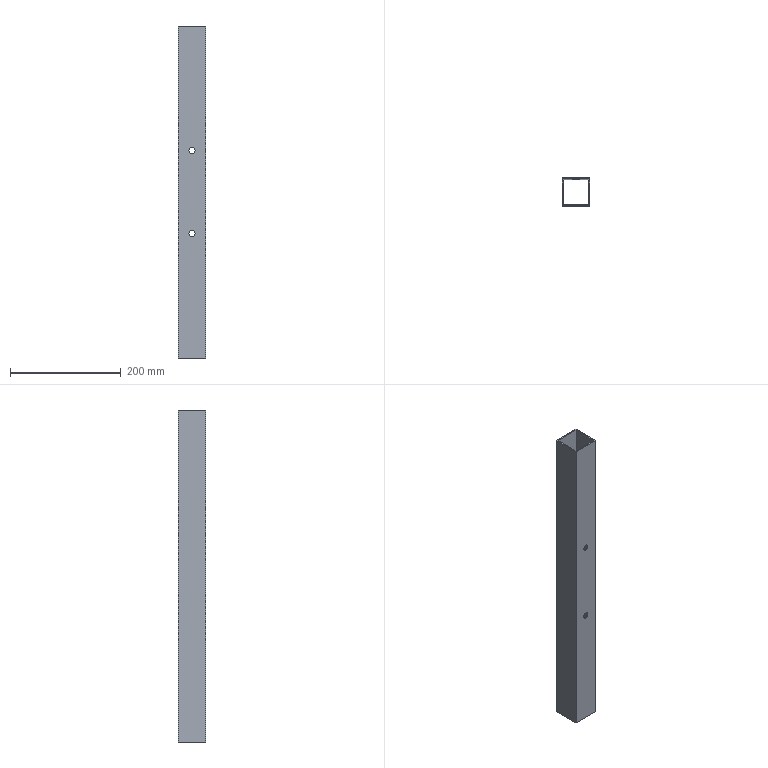Part | SolidWorks | features Cut 1, Extrusion 1 | 1 solid | 18 faces | box 50 x 50 x 600 mm | volume 229640 mm3 | plane 10 | cylinder 8 | commonest cylinder face diameters 11 x8
STEP:
#1=CARTESIAN_POINT('',(0.,23.,380.5));
#2=VERTEX_POINT('',#1);
#3=CARTESIAN_POINT('',(0.,23.,369.5));
#4=VERTEX_POINT('',#3);
#5=CARTESIAN_POINT('',(0.,23.,375.));
#6=DIRECTION('',(0.,-1.,0.));
#7=DIRECTION('',(0.,0.,-1.));
#8=AXIS2_PLACEMENT_3D('',#5,#6,#7);
#9=CIRCLE('',#8,5.5);
#10=EDGE_CURVE('',#2,#4,#9,.T.);
#11=ORIENTED_EDGE('',*,*,#10,.T.);
#12=CARTESIAN_POINT('',(0.,25.,369.5));
#13=VERTEX_POINT('',#12);
#14=CARTESIAN_POINT('',(0.,-25.,369.5));
#15=DIRECTION('',(0.,1.,0.));
#16=VECTOR('',#15,1000.);
#17=LINE('',#14,#16);
#18=EDGE_CURVE('',#4,#13,#17,.T.);
#19=ORIENTED_EDGE('',*,*,#18,.T.);
#20=CARTESIAN_POINT('',(0.,25.,380.5));
#21=VERTEX_POINT('',#20);
#22=CARTESIAN_POINT('',(0.,25.,375.));
#23=DIRECTION('',(0.,1.,0.));
#24=DIRECTION('',(0.,0.,1.));
#25=AXIS2_PLACEMENT_3D('',#22,#23,#24);
#26=CIRCLE('',#25,5.5);
#27=EDGE_CURVE('',#13,#21,#26,.T.);
#28=ORIENTED_EDGE('',*,*,#27,.T.);
#29=CARTESIAN_POINT('',(0.,-25.,380.5));
#30=DIRECTION('',(0.,1.,0.));
#31=VECTOR('',#30,1000.);
#32=LINE('',#29,#31);
#33=EDGE_CURVE('',#2,#21,#32,.T.);
#34=ORIENTED_EDGE('',*,*,#33,.F.);
#35=EDGE_LOOP('',(#11,#19,#28,#34));
#36=FACE_OUTER_BOUND('',#35,.T.);
#37=CARTESIAN_POINT('',(0.,-25.,375.));
#38=DIRECTION('',(0.,1.,0.));
#39=DIRECTION('',(0.,0.,1.));
#40=AXIS2_PLACEMENT_3D('',#37,#38,#39);
#41=CYLINDRICAL_SURFACE('',#40,5.5);
#42=ADVANCED_FACE('',(#36),#41,.F.);
#43=CARTESIAN_POINT('',(0.,-25.,369.5));
#44=VERTEX_POINT('',#43);
#45=CARTESIAN_POINT('',(0.,-25.,380.5));
#46=VERTEX_POINT('',#45);
#47=CARTESIAN_POINT('',(0.,-25.,375.));
#48=DIRECTION('',(0.,1.,0.));
#49=DIRECTION('',(0.,0.,1.));
#50=AXIS2_PLACEMENT_3D('',#47,#48,#49);
#51=CIRCLE('',#50,5.5);
#52=EDGE_CURVE('',#44,#46,#51,.T.);
#53=ORIENTED_EDGE('',*,*,#52,.F.);
#54=CARTESIAN_POINT('',(0.,-23.,369.5));
#55=VERTEX_POINT('',#54);
#56=CARTESIAN_POINT('',(0.,-25.,369.5));
#57=DIRECTION('',(0.,1.,0.));
#58=VECTOR('',#57,1000.);
#59=LINE('',#56,#58);
#60=EDGE_CURVE('',#44,#55,#59,.T.);
#61=ORIENTED_EDGE('',*,*,#60,.T.);
#62=CARTESIAN_POINT('',(0.,-23.,380.5));
#63=VERTEX_POINT('',#62);
#64=CARTESIAN_POINT('',(0.,-23.,375.));
#65=DIRECTION('',(0.,1.,0.));
#66=DIRECTION('',(0.,0.,1.));
#67=AXIS2_PLACEMENT_3D('',#64,#65,#66);
#68=CIRCLE('',#67,5.5);
#69=EDGE_CURVE('',#55,#63,#68,.T.);
#70=ORIENTED_EDGE('',*,*,#69,.T.);
#71=CARTESIAN_POINT('',(0.,-25.,380.5));
#72=DIRECTION('',(0.,1.,0.));
#73=VECTOR('',#72,1000.);
#74=LINE('',#71,#73);
#75=EDGE_CURVE('',#46,#63,#74,.T.);
#76=ORIENTED_EDGE('',*,*,#75,.F.);
#77=EDGE_LOOP('',(#53,#61,#70,#76));
#78=FACE_OUTER_BOUND('',#77,.T.);
#79=CARTESIAN_POINT('',(0.,-25.,375.));
#80=DIRECTION('',(0.,1.,0.));
#81=DIRECTION('',(0.,0.,1.));
#82=AXIS2_PLACEMENT_3D('',#79,#80,#81);
#83=CYLINDRICAL_SURFACE('',#82,5.5);
#84=ADVANCED_FACE('',(#78),#83,.F.);
#85=CARTESIAN_POINT('',(0.,23.,230.5));
#86=VERTEX_POINT('',#85);
#87=CARTESIAN_POINT('',(0.,23.,219.5));
#88=VERTEX_POINT('',#87);
#89=CARTESIAN_POINT('',(0.,23.,225.));
#90=DIRECTION('',(0.,-1.,0.));
#91=DIRECTION('',(0.,0.,-1.));
#92=AXIS2_PLACEMENT_3D('',#89,#90,#91);
#93=CIRCLE('',#92,5.5);
#94=EDGE_CURVE('',#86,#88,#93,.T.);
#95=ORIENTED_EDGE('',*,*,#94,.T.);
#96=CARTESIAN_POINT('',(0.,25.,219.5));
#97=VERTEX_POINT('',#96);
#98=CARTESIAN_POINT('',(0.,-25.,219.5));
#99=DIRECTION('',(0.,1.,0.));
#100=VECTOR('',#99,1000.);
#101=LINE('',#98,#100);
#102=EDGE_CURVE('',#88,#97,#101,.T.);
#103=ORIENTED_EDGE('',*,*,#102,.T.);
#104=CARTESIAN_POINT('',(0.,25.,230.5));
#105=VERTEX_POINT('',#104);
#106=CARTESIAN_POINT('',(0.,25.,225.));
#107=DIRECTION('',(0.,1.,0.));
#108=DIRECTION('',(0.,0.,1.));
#109=AXIS2_PLACEMENT_3D('',#106,#107,#108);
#110=CIRCLE('',#109,5.5);
#111=EDGE_CURVE('',#97,#105,#110,.T.);
#112=ORIENTED_EDGE('',*,*,#111,.T.);
#113=CARTESIAN_POINT('',(0.,-25.,230.5));
#114=DIRECTION('',(0.,1.,0.));
#115=VECTOR('',#114,1000.);
#116=LINE('',#113,#115);
#117=EDGE_CURVE('',#86,#105,#116,.T.);
#118=ORIENTED_EDGE('',*,*,#117,.F.);
#119=EDGE_LOOP('',(#95,#103,#112,#118));
#120=FACE_OUTER_BOUND('',#119,.T.);
#121=CARTESIAN_POINT('',(0.,-25.,225.));
#122=DIRECTION('',(0.,1.,0.));
#123=DIRECTION('',(0.,0.,1.));
#124=AXIS2_PLACEMENT_3D('',#121,#122,#123);
#125=CYLINDRICAL_SURFACE('',#124,5.5);
#126=ADVANCED_FACE('',(#120),#125,.F.);
#127=CARTESIAN_POINT('',(0.,-25.,219.5));
#128=VERTEX_POINT('',#127);
#129=CARTESIAN_POINT('',(0.,-25.,230.5));
#130=VERTEX_POINT('',#129);
#131=CARTESIAN_POINT('',(0.,-25.,225.));
#132=DIRECTION('',(0.,1.,0.));
#133=DIRECTION('',(0.,0.,1.));
#134=AXIS2_PLACEMENT_3D('',#131,#132,#133);
#135=CIRCLE('',#134,5.5);
#136=EDGE_CURVE('',#128,#130,#135,.T.);
#137=ORIENTED_EDGE('',*,*,#136,.F.);
#138=CARTESIAN_POINT('',(0.,-23.,219.5));
#139=VERTEX_POINT('',#138);
#140=CARTESIAN_POINT('',(0.,-25.,219.5));
#141=DIRECTION('',(0.,1.,0.));
#142=VECTOR('',#141,1000.);
#143=LINE('',#140,#142);
#144=EDGE_CURVE('',#128,#139,#143,.T.);
#145=ORIENTED_EDGE('',*,*,#144,.T.);
#146=CARTESIAN_POINT('',(0.,-23.,230.5));
#147=VERTEX_POINT('',#146);
#148=CARTESIAN_POINT('',(0.,-23.,225.));
#149=DIRECTION('',(0.,1.,0.));
#150=DIRECTION('',(0.,0.,1.));
#151=AXIS2_PLACEMENT_3D('',#148,#149,#150);
#152=CIRCLE('',#151,5.5);
#153=EDGE_CURVE('',#139,#147,#152,.T.);
#154=ORIENTED_EDGE('',*,*,#153,.T.);
#155=CARTESIAN_POINT('',(0.,-25.,230.5));
#156=DIRECTION('',(0.,1.,0.));
#157=VECTOR('',#156,1000.);
#158=LINE('',#155,#157);
#159=EDGE_CURVE('',#130,#147,#158,.T.);
#160=ORIENTED_EDGE('',*,*,#159,.F.);
#161=EDGE_LOOP('',(#137,#145,#154,#160));
#162=FACE_OUTER_BOUND('',#161,.T.);
#163=CARTESIAN_POINT('',(0.,-25.,225.));
#164=DIRECTION('',(0.,1.,0.));
#165=DIRECTION('',(0.,0.,1.));
#166=AXIS2_PLACEMENT_3D('',#163,#164,#165);
#167=CYLINDRICAL_SURFACE('',#166,5.5);
#168=ADVANCED_FACE('',(#162),#167,.F.);
#169=CARTESIAN_POINT('',(25.,-25.,600.));
#170=VERTEX_POINT('',#169);
#171=CARTESIAN_POINT('',(25.,25.,600.));
#172=VERTEX_POINT('',#171);
#173=CARTESIAN_POINT('',(25.,-25.,600.));
#174=DIRECTION('',(0.,1.,0.));
#175=VECTOR('',#174,1000.);
#176=LINE('',#173,#175);
#177=EDGE_CURVE('',#170,#172,#176,.T.);
#178=ORIENTED_EDGE('',*,*,#177,.T.);
#179=CARTESIAN_POINT('',(-25.,25.,600.));
#180=VERTEX_POINT('',#179);
#181=CARTESIAN_POINT('',(-25.,25.,600.));
#182=DIRECTION('',(-1.,0.,0.));
#183=VECTOR('',#182,1000.);
#184=LINE('',#181,#183);
#185=EDGE_CURVE('',#172,#180,#184,.T.);
#186=ORIENTED_EDGE('',*,*,#185,.T.);
#187=CARTESIAN_POINT('',(-25.,-25.,600.));
#188=VERTEX_POINT('',#187);
#189=CARTESIAN_POINT('',(-25.,-25.,600.));
#190=DIRECTION('',(0.,-1.,0.));
#191=VECTOR('',#190,1000.);
#192=LINE('',#189,#191);
#193=EDGE_CURVE('',#180,#188,#192,.T.);
#194=ORIENTED_EDGE('',*,*,#193,.T.);
#195=CARTESIAN_POINT('',(-25.,-25.,600.));
#196=DIRECTION('',(1.,0.,0.));
#197=VECTOR('',#196,1000.);
#198=LINE('',#195,#197);
#199=EDGE_CURVE('',#188,#170,#198,.T.);
#200=ORIENTED_EDGE('',*,*,#199,.T.);
#201=EDGE_LOOP('',(#178,#186,#194,#200));
#202=FACE_OUTER_BOUND('',#201,.T.);
#203=CARTESIAN_POINT('',(23.,-23.,600.));
#204=VERTEX_POINT('',#203);
#205=CARTESIAN_POINT('',(23.,23.,600.));
#206=VERTEX_POINT('',#205);
#207=CARTESIAN_POINT('',(23.,-23.,600.));
#208=DIRECTION('',(0.,1.,0.));
#209=VECTOR('',#208,1000.);
#210=LINE('',#207,#209);
#211=EDGE_CURVE('',#204,#206,#210,.T.);
#212=ORIENTED_EDGE('',*,*,#211,.F.);
#213=CARTESIAN_POINT('',(-23.,-23.,600.));
#214=VERTEX_POINT('',#213);
#215=CARTESIAN_POINT('',(-23.,-23.,600.));
#216=DIRECTION('',(1.,0.,0.));
#217=VECTOR('',#216,1000.);
#218=LINE('',#215,#217);
#219=EDGE_CURVE('',#214,#204,#218,.T.);
#220=ORIENTED_EDGE('',*,*,#219,.F.);
#221=CARTESIAN_POINT('',(-23.,23.,600.));
#222=VERTEX_POINT('',#221);
#223=CARTESIAN_POINT('',(-23.,-23.,600.));
#224=DIRECTION('',(0.,-1.,0.));
#225=VECTOR('',#224,1000.);
#226=LINE('',#223,#225);
#227=EDGE_CURVE('',#222,#214,#226,.T.);
#228=ORIENTED_EDGE('',*,*,#227,.F.);
#229=CARTESIAN_POINT('',(-23.,23.,600.));
#230=DIRECTION('',(-1.,0.,0.));
#231=VECTOR('',#230,1000.);
#232=LINE('',#229,#231);
#233=EDGE_CURVE('',#206,#222,#232,.T.);
#234=ORIENTED_EDGE('',*,*,#233,.F.);
#235=EDGE_LOOP('',(#212,#220,#228,#234));
#236=FACE_BOUND('',#235,.T.);
#237=CARTESIAN_POINT('',(0.,0.,600.));
#238=DIRECTION('',(0.,0.,-1.));
#239=DIRECTION('',(-1.,0.,0.));
#240=AXIS2_PLACEMENT_3D('',#237,#238,#239);
#241=PLANE('',#240);
#242=ADVANCED_FACE('',(#202,#236),#241,.F.);
#243=CARTESIAN_POINT('',(25.,-25.,0.));
#244=VERTEX_POINT('',#243);
#245=CARTESIAN_POINT('',(25.,25.,0.));
#246=VERTEX_POINT('',#245);
#247=CARTESIAN_POINT('',(25.,-25.,0.));
#248=DIRECTION('',(0.,1.,0.));
#249=VECTOR('',#248,1000.);
#250=LINE('',#247,#249);
#251=EDGE_CURVE('',#244,#246,#250,.T.);
#252=ORIENTED_EDGE('',*,*,#251,.F.);
#253=CARTESIAN_POINT('',(-25.,-25.,0.));
#254=VERTEX_POINT('',#253);
#255=CARTESIAN_POINT('',(-25.,-25.,0.));
#256=DIRECTION('',(1.,0.,0.));
#257=VECTOR('',#256,1000.);
#258=LINE('',#255,#257);
#259=EDGE_CURVE('',#254,#244,#258,.T.);
#260=ORIENTED_EDGE('',*,*,#259,.F.);
#261=CARTESIAN_POINT('',(-25.,25.,0.));
#262=VERTEX_POINT('',#261);
#263=CARTESIAN_POINT('',(-25.,-25.,0.));
#264=DIRECTION('',(0.,-1.,0.));
#265=VECTOR('',#264,1000.);
#266=LINE('',#263,#265);
#267=EDGE_CURVE('',#262,#254,#266,.T.);
#268=ORIENTED_EDGE('',*,*,#267,.F.);
#269=CARTESIAN_POINT('',(-25.,25.,0.));
#270=DIRECTION('',(-1.,0.,0.));
#271=VECTOR('',#270,1000.);
#272=LINE('',#269,#271);
#273=EDGE_CURVE('',#246,#262,#272,.T.);
#274=ORIENTED_EDGE('',*,*,#273,.F.);
#275=EDGE_LOOP('',(#252,#260,#268,#274));
#276=FACE_OUTER_BOUND('',#275,.T.);
#277=CARTESIAN_POINT('',(-23.,-23.,0.));
#278=VERTEX_POINT('',#277);
#279=CARTESIAN_POINT('',(23.,-23.,0.));
#280=VERTEX_POINT('',#279);
#281=CARTESIAN_POINT('',(-23.,-23.,0.));
#282=DIRECTION('',(1.,0.,0.));
#283=VECTOR('',#282,1000.);
#284=LINE('',#281,#283);
#285=EDGE_CURVE('',#278,#280,#284,.T.);
#286=ORIENTED_EDGE('',*,*,#285,.T.);
#287=CARTESIAN_POINT('',(23.,23.,0.));
#288=VERTEX_POINT('',#287);
#289=CARTESIAN_POINT('',(23.,-23.,0.));
#290=DIRECTION('',(0.,1.,0.));
#291=VECTOR('',#290,1000.);
#292=LINE('',#289,#291);
#293=EDGE_CURVE('',#280,#288,#292,.T.);
#294=ORIENTED_EDGE('',*,*,#293,.T.);
#295=CARTESIAN_POINT('',(-23.,23.,0.));
#296=VERTEX_POINT('',#295);
#297=CARTESIAN_POINT('',(-23.,23.,0.));
#298=DIRECTION('',(-1.,0.,0.));
#299=VECTOR('',#298,1000.);
#300=LINE('',#297,#299);
#301=EDGE_CURVE('',#288,#296,#300,.T.);
#302=ORIENTED_EDGE('',*,*,#301,.T.);
#303=CARTESIAN_POINT('',(-23.,-23.,0.));
#304=DIRECTION('',(0.,-1.,0.));
#305=VECTOR('',#304,1000.);
#306=LINE('',#303,#305);
#307=EDGE_CURVE('',#296,#278,#306,.T.);
#308=ORIENTED_EDGE('',*,*,#307,.T.);
#309=EDGE_LOOP('',(#286,#294,#302,#308));
#310=FACE_BOUND('',#309,.T.);
#311=CARTESIAN_POINT('',(0.,0.,0.));
#312=DIRECTION('',(0.,0.,-1.));
#313=DIRECTION('',(-1.,0.,0.));
#314=AXIS2_PLACEMENT_3D('',#311,#312,#313);
#315=PLANE('',#314);
#316=ADVANCED_FACE('',(#276,#310),#315,.T.);
#317=ORIENTED_EDGE('',*,*,#251,.T.);
#318=CARTESIAN_POINT('',(25.,25.,600.));
#319=DIRECTION('',(0.,0.,-1.));
#320=VECTOR('',#319,1000.);
#321=LINE('',#318,#320);
#322=EDGE_CURVE('',#172,#246,#321,.T.);
#323=ORIENTED_EDGE('',*,*,#322,.F.);
#324=ORIENTED_EDGE('',*,*,#177,.F.);
#325=CARTESIAN_POINT('',(25.,-25.,600.));
#326=DIRECTION('',(0.,0.,-1.));
#327=VECTOR('',#326,1000.);
#328=LINE('',#325,#327);
#329=EDGE_CURVE('',#170,#244,#328,.T.);
#330=ORIENTED_EDGE('',*,*,#329,.T.);
#331=EDGE_LOOP('',(#317,#323,#324,#330));
#332=FACE_OUTER_BOUND('',#331,.T.);
#333=CARTESIAN_POINT('',(25.,-25.,600.));
#334=DIRECTION('',(-1.,0.,0.));
#335=DIRECTION('',(0.,0.,1.));
#336=AXIS2_PLACEMENT_3D('',#333,#334,#335);
#337=PLANE('',#336);
#338=ADVANCED_FACE('',(#332),#337,.F.);
#339=CARTESIAN_POINT('',(0.,25.,375.));
#340=DIRECTION('',(0.,1.,0.));
#341=DIRECTION('',(0.,0.,1.));
#342=AXIS2_PLACEMENT_3D('',#339,#340,#341);
#343=CIRCLE('',#342,5.5);
#344=EDGE_CURVE('',#21,#13,#343,.T.);
#345=ORIENTED_EDGE('',*,*,#344,.F.);
#346=ORIENTED_EDGE('',*,*,#27,.F.);
#347=EDGE_LOOP('',(#345,#346));
#348=FACE_BOUND('',#347,.T.);
#349=CARTESIAN_POINT('',(0.,25.,225.));
#350=DIRECTION('',(0.,1.,0.));
#351=DIRECTION('',(0.,0.,1.));
#352=AXIS2_PLACEMENT_3D('',#349,#350,#351);
#353=CIRCLE('',#352,5.5);
#354=EDGE_CURVE('',#105,#97,#353,.T.);
#355=ORIENTED_EDGE('',*,*,#354,.F.);
#356=ORIENTED_EDGE('',*,*,#111,.F.);
#357=EDGE_LOOP('',(#355,#356));
#358=FACE_BOUND('',#357,.T.);
#359=ORIENTED_EDGE('',*,*,#273,.T.);
#360=CARTESIAN_POINT('',(-25.,25.,600.));
#361=DIRECTION('',(0.,0.,-1.));
#362=VECTOR('',#361,1000.);
#363=LINE('',#360,#362);
#364=EDGE_CURVE('',#180,#262,#363,.T.);
#365=ORIENTED_EDGE('',*,*,#364,.F.);
#366=ORIENTED_EDGE('',*,*,#185,.F.);
#367=ORIENTED_EDGE('',*,*,#322,.T.);
#368=EDGE_LOOP('',(#359,#365,#366,#367));
#369=FACE_OUTER_BOUND('',#368,.T.);
#370=CARTESIAN_POINT('',(-25.,25.,600.));
#371=DIRECTION('',(0.,-1.,0.));
#372=DIRECTION('',(0.,0.,-1.));
#373=AXIS2_PLACEMENT_3D('',#370,#371,#372);
#374=PLANE('',#373);
#375=ADVANCED_FACE('',(#348,#358,#369),#374,.F.);
#376=ORIENTED_EDGE('',*,*,#267,.T.);
#377=CARTESIAN_POINT('',(-25.,-25.,600.));
#378=DIRECTION('',(0.,0.,-1.));
#379=VECTOR('',#378,1000.);
#380=LINE('',#377,#379);
#381=EDGE_CURVE('',#188,#254,#380,.T.);
#382=ORIENTED_EDGE('',*,*,#381,.F.);
#383=ORIENTED_EDGE('',*,*,#193,.F.);
#384=ORIENTED_EDGE('',*,*,#364,.T.);
#385=EDGE_LOOP('',(#376,#382,#383,#384));
#386=FACE_OUTER_BOUND('',#385,.T.);
#387=CARTESIAN_POINT('',(-25.,-25.,600.));
#388=DIRECTION('',(1.,0.,0.));
#389=DIRECTION('',(0.,0.,-1.));
#390=AXIS2_PLACEMENT_3D('',#387,#388,#389);
#391=PLANE('',#390);
#392=ADVANCED_FACE('',(#386),#391,.F.);
#393=CARTESIAN_POINT('',(0.,-25.,375.));
#394=DIRECTION('',(0.,1.,0.));
#395=DIRECTION('',(0.,0.,1.));
#396=AXIS2_PLACEMENT_3D('',#393,#394,#395);
#397=CIRCLE('',#396,5.5);
#398=EDGE_CURVE('',#46,#44,#397,.T.);
#399=ORIENTED_EDGE('',*,*,#398,.T.);
#400=ORIENTED_EDGE('',*,*,#52,.T.);
#401=EDGE_LOOP('',(#399,#400));
#402=FACE_BOUND('',#401,.T.);
#403=CARTESIAN_POINT('',(0.,-25.,225.));
#404=DIRECTION('',(0.,1.,0.));
#405=DIRECTION('',(0.,0.,1.));
#406=AXIS2_PLACEMENT_3D('',#403,#404,#405);
#407=CIRCLE('',#406,5.5);
#408=EDGE_CURVE('',#130,#128,#407,.T.);
#409=ORIENTED_EDGE('',*,*,#408,.T.);
#410=ORIENTED_EDGE('',*,*,#136,.T.);
#411=EDGE_LOOP('',(#409,#410));
#412=FACE_BOUND('',#411,.T.);
#413=ORIENTED_EDGE('',*,*,#259,.T.);
#414=ORIENTED_EDGE('',*,*,#329,.F.);
#415=ORIENTED_EDGE('',*,*,#199,.F.);
#416=ORIENTED_EDGE('',*,*,#381,.T.);
#417=EDGE_LOOP('',(#413,#414,#415,#416));
#418=FACE_OUTER_BOUND('',#417,.T.);
#419=CARTESIAN_POINT('',(-25.,-25.,600.));
#420=DIRECTION('',(0.,1.,0.));
#421=DIRECTION('',(0.,0.,1.));
#422=AXIS2_PLACEMENT_3D('',#419,#420,#421);
#423=PLANE('',#422);
#424=ADVANCED_FACE('',(#402,#412,#418),#423,.F.);
#425=ORIENTED_EDGE('',*,*,#293,.F.);
#426=CARTESIAN_POINT('',(23.,-23.,600.));
#427=DIRECTION('',(0.,0.,-1.));
#428=VECTOR('',#427,1000.);
#429=LINE('',#426,#428);
#430=EDGE_CURVE('',#204,#280,#429,.T.);
#431=ORIENTED_EDGE('',*,*,#430,.F.);
#432=ORIENTED_EDGE('',*,*,#211,.T.);
#433=CARTESIAN_POINT('',(23.,23.,600.));
#434=DIRECTION('',(0.,0.,-1.));
#435=VECTOR('',#434,1000.);
#436=LINE('',#433,#435);
#437=EDGE_CURVE('',#206,#288,#436,.T.);
#438=ORIENTED_EDGE('',*,*,#437,.T.);
#439=EDGE_LOOP('',(#425,#431,#432,#438));
#440=FACE_OUTER_BOUND('',#439,.T.);
#441=CARTESIAN_POINT('',(23.,-23.,600.));
#442=DIRECTION('',(-1.,0.,0.));
#443=DIRECTION('',(0.,0.,1.));
#444=AXIS2_PLACEMENT_3D('',#441,#442,#443);
#445=PLANE('',#444);
#446=ADVANCED_FACE('',(#440),#445,.T.);
#447=ORIENTED_EDGE('',*,*,#10,.F.);
#448=CARTESIAN_POINT('',(0.,23.,375.));
#449=DIRECTION('',(0.,-1.,0.));
#450=DIRECTION('',(0.,0.,-1.));
#451=AXIS2_PLACEMENT_3D('',#448,#449,#450);
#452=CIRCLE('',#451,5.5);
#453=EDGE_CURVE('',#4,#2,#452,.T.);
#454=ORIENTED_EDGE('',*,*,#453,.F.);
#455=EDGE_LOOP('',(#447,#454));
#456=FACE_BOUND('',#455,.T.);
#457=ORIENTED_EDGE('',*,*,#94,.F.);
#458=CARTESIAN_POINT('',(0.,23.,225.));
#459=DIRECTION('',(0.,-1.,0.));
#460=DIRECTION('',(0.,0.,-1.));
#461=AXIS2_PLACEMENT_3D('',#458,#459,#460);
#462=CIRCLE('',#461,5.5);
#463=EDGE_CURVE('',#88,#86,#462,.T.);
#464=ORIENTED_EDGE('',*,*,#463,.F.);
#465=EDGE_LOOP('',(#457,#464));
#466=FACE_BOUND('',#465,.T.);
#467=ORIENTED_EDGE('',*,*,#301,.F.);
#468=ORIENTED_EDGE('',*,*,#437,.F.);
#469=ORIENTED_EDGE('',*,*,#233,.T.);
#470=CARTESIAN_POINT('',(-23.,23.,600.));
#471=DIRECTION('',(0.,0.,-1.));
#472=VECTOR('',#471,1000.);
#473=LINE('',#470,#472);
#474=EDGE_CURVE('',#222,#296,#473,.T.);
#475=ORIENTED_EDGE('',*,*,#474,.T.);
#476=EDGE_LOOP('',(#467,#468,#469,#475));
#477=FACE_OUTER_BOUND('',#476,.T.);
#478=CARTESIAN_POINT('',(-23.,23.,600.));
#479=DIRECTION('',(0.,-1.,0.));
#480=DIRECTION('',(0.,0.,-1.));
#481=AXIS2_PLACEMENT_3D('',#478,#479,#480);
#482=PLANE('',#481);
#483=ADVANCED_FACE('',(#456,#466,#477),#482,.T.);
#484=ORIENTED_EDGE('',*,*,#307,.F.);
#485=ORIENTED_EDGE('',*,*,#474,.F.);
#486=ORIENTED_EDGE('',*,*,#227,.T.);
#487=CARTESIAN_POINT('',(-23.,-23.,600.));
#488=DIRECTION('',(0.,0.,-1.));
#489=VECTOR('',#488,1000.);
#490=LINE('',#487,#489);
#491=EDGE_CURVE('',#214,#278,#490,.T.);
#492=ORIENTED_EDGE('',*,*,#491,.T.);
#493=EDGE_LOOP('',(#484,#485,#486,#492));
#494=FACE_OUTER_BOUND('',#493,.T.);
#495=CARTESIAN_POINT('',(-23.,-23.,600.));
#496=DIRECTION('',(1.,0.,0.));
#497=DIRECTION('',(0.,0.,-1.));
#498=AXIS2_PLACEMENT_3D('',#495,#496,#497);
#499=PLANE('',#498);
#500=ADVANCED_FACE('',(#494),#499,.T.);
#501=CARTESIAN_POINT('',(0.,-23.,375.));
#502=DIRECTION('',(0.,1.,0.));
#503=DIRECTION('',(0.,0.,1.));
#504=AXIS2_PLACEMENT_3D('',#501,#502,#503);
#505=CIRCLE('',#504,5.5);
#506=EDGE_CURVE('',#63,#55,#505,.T.);
#507=ORIENTED_EDGE('',*,*,#506,.F.);
#508=ORIENTED_EDGE('',*,*,#69,.F.);
#509=EDGE_LOOP('',(#507,#508));
#510=FACE_BOUND('',#509,.T.);
#511=CARTESIAN_POINT('',(0.,-23.,225.));
#512=DIRECTION('',(0.,1.,0.));
#513=DIRECTION('',(0.,0.,1.));
#514=AXIS2_PLACEMENT_3D('',#511,#512,#513);
#515=CIRCLE('',#514,5.5);
#516=EDGE_CURVE('',#147,#139,#515,.T.);
#517=ORIENTED_EDGE('',*,*,#516,.F.);
#518=ORIENTED_EDGE('',*,*,#153,.F.);
#519=EDGE_LOOP('',(#517,#518));
#520=FACE_BOUND('',#519,.T.);
#521=ORIENTED_EDGE('',*,*,#285,.F.);
#522=ORIENTED_EDGE('',*,*,#491,.F.);
#523=ORIENTED_EDGE('',*,*,#219,.T.);
#524=ORIENTED_EDGE('',*,*,#430,.T.);
#525=EDGE_LOOP('',(#521,#522,#523,#524));
#526=FACE_OUTER_BOUND('',#525,.T.);
#527=CARTESIAN_POINT('',(-23.,-23.,600.));
#528=DIRECTION('',(0.,1.,0.));
#529=DIRECTION('',(0.,0.,1.));
#530=AXIS2_PLACEMENT_3D('',#527,#528,#529);
#531=PLANE('',#530);
#532=ADVANCED_FACE('',(#510,#520,#526),#531,.T.);
#533=ORIENTED_EDGE('',*,*,#144,.F.);
#534=ORIENTED_EDGE('',*,*,#408,.F.);
#535=ORIENTED_EDGE('',*,*,#159,.T.);
#536=ORIENTED_EDGE('',*,*,#516,.T.);
#537=EDGE_LOOP('',(#533,#534,#535,#536));
#538=FACE_OUTER_BOUND('',#537,.T.);
#539=CARTESIAN_POINT('',(0.,-25.,225.));
#540=DIRECTION('',(0.,1.,0.));
#541=DIRECTION('',(0.,0.,1.));
#542=AXIS2_PLACEMENT_3D('',#539,#540,#541);
#543=CYLINDRICAL_SURFACE('',#542,5.5);
#544=ADVANCED_FACE('',(#538),#543,.F.);
#545=ORIENTED_EDGE('',*,*,#102,.F.);
#546=ORIENTED_EDGE('',*,*,#463,.T.);
#547=ORIENTED_EDGE('',*,*,#117,.T.);
#548=ORIENTED_EDGE('',*,*,#354,.T.);
#549=EDGE_LOOP('',(#545,#546,#547,#548));
#550=FACE_OUTER_BOUND('',#549,.T.);
#551=CARTESIAN_POINT('',(0.,-25.,225.));
#552=DIRECTION('',(0.,1.,0.));
#553=DIRECTION('',(0.,0.,1.));
#554=AXIS2_PLACEMENT_3D('',#551,#552,#553);
#555=CYLINDRICAL_SURFACE('',#554,5.5);
#556=ADVANCED_FACE('',(#550),#555,.F.);
#557=ORIENTED_EDGE('',*,*,#60,.F.);
#558=ORIENTED_EDGE('',*,*,#398,.F.);
#559=ORIENTED_EDGE('',*,*,#75,.T.);
#560=ORIENTED_EDGE('',*,*,#506,.T.);
#561=EDGE_LOOP('',(#557,#558,#559,#560));
#562=FACE_OUTER_BOUND('',#561,.T.);
#563=CARTESIAN_POINT('',(0.,-25.,375.));
#564=DIRECTION('',(0.,1.,0.));
#565=DIRECTION('',(0.,0.,1.));
#566=AXIS2_PLACEMENT_3D('',#563,#564,#565);
#567=CYLINDRICAL_SURFACE('',#566,5.5);
#568=ADVANCED_FACE('',(#562),#567,.F.);
#569=ORIENTED_EDGE('',*,*,#18,.F.);
#570=ORIENTED_EDGE('',*,*,#453,.T.);
#571=ORIENTED_EDGE('',*,*,#33,.T.);
#572=ORIENTED_EDGE('',*,*,#344,.T.);
#573=EDGE_LOOP('',(#569,#570,#571,#572));
#574=FACE_OUTER_BOUND('',#573,.T.);
#575=CARTESIAN_POINT('',(0.,-25.,375.));
#576=DIRECTION('',(0.,1.,0.));
#577=DIRECTION('',(0.,0.,1.));
#578=AXIS2_PLACEMENT_3D('',#575,#576,#577);
#579=CYLINDRICAL_SURFACE('',#578,5.5);
#580=ADVANCED_FACE('',(#574),#579,.F.);
#581=CLOSED_SHELL('',(#42,#84,#126,#168,#242,#316,#338,#375,#392,#424,#446,#483,#500,#532,#544,#556,#568,#580));
#582=MANIFOLD_SOLID_BREP('',#581);
#583=CARTESIAN_POINT('',(0.,0.,0.));
#584=DIRECTION('',(0.,0.,1.));
#585=DIRECTION('',(1.,0.,0.));
#586=AXIS2_PLACEMENT_3D('',#583,#584,#585);
#587=(LENGTH_UNIT()NAMED_UNIT(*)SI_UNIT(.MILLI.,.METRE.));
#588=UNCERTAINTY_MEASURE_WITH_UNIT(LENGTH_MEASURE(0.00001),#587,'','');
#589=(NAMED_UNIT(*)PLANE_ANGLE_UNIT()SI_UNIT($,.RADIAN.));
#590=(NAMED_UNIT(*)SI_UNIT($,.STERADIAN.)SOLID_ANGLE_UNIT());
#591=(GEOMETRIC_REPRESENTATION_CONTEXT(3)GLOBAL_UNCERTAINTY_ASSIGNED_CONTEXT((#588))GLOBAL_UNIT_ASSIGNED_CONTEXT((#587,#589,#590))REPRESENTATION_CONTEXT('',''));
#592=ADVANCED_BREP_SHAPE_REPRESENTATION('',(#582,#586),#591);